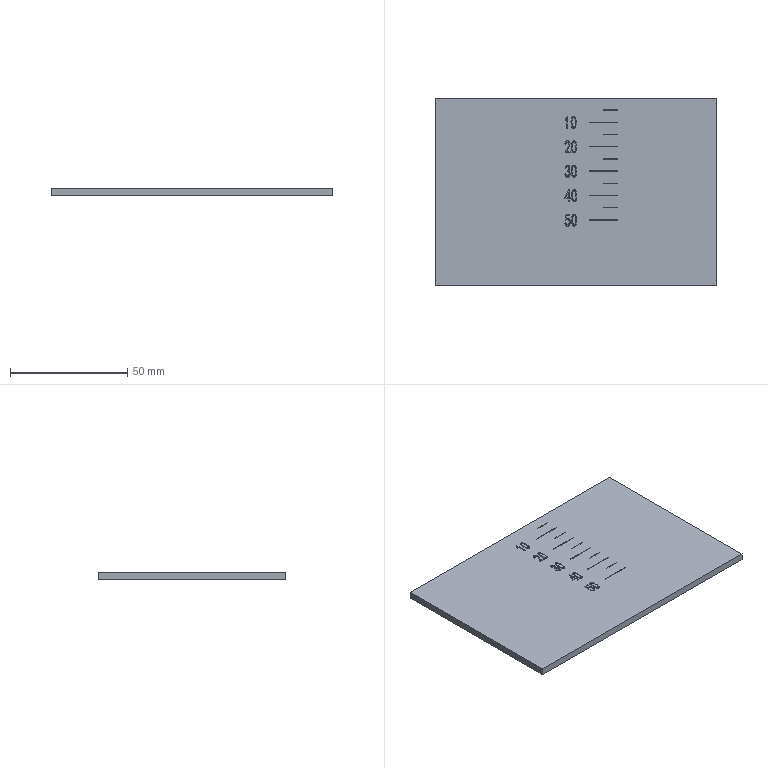Part | SolidWorks | features BaseBody 1 | 1 solid | 141 faces | box 120 x 80 x 3 mm | volume 28774 mm3 | plane 104 | spline 37